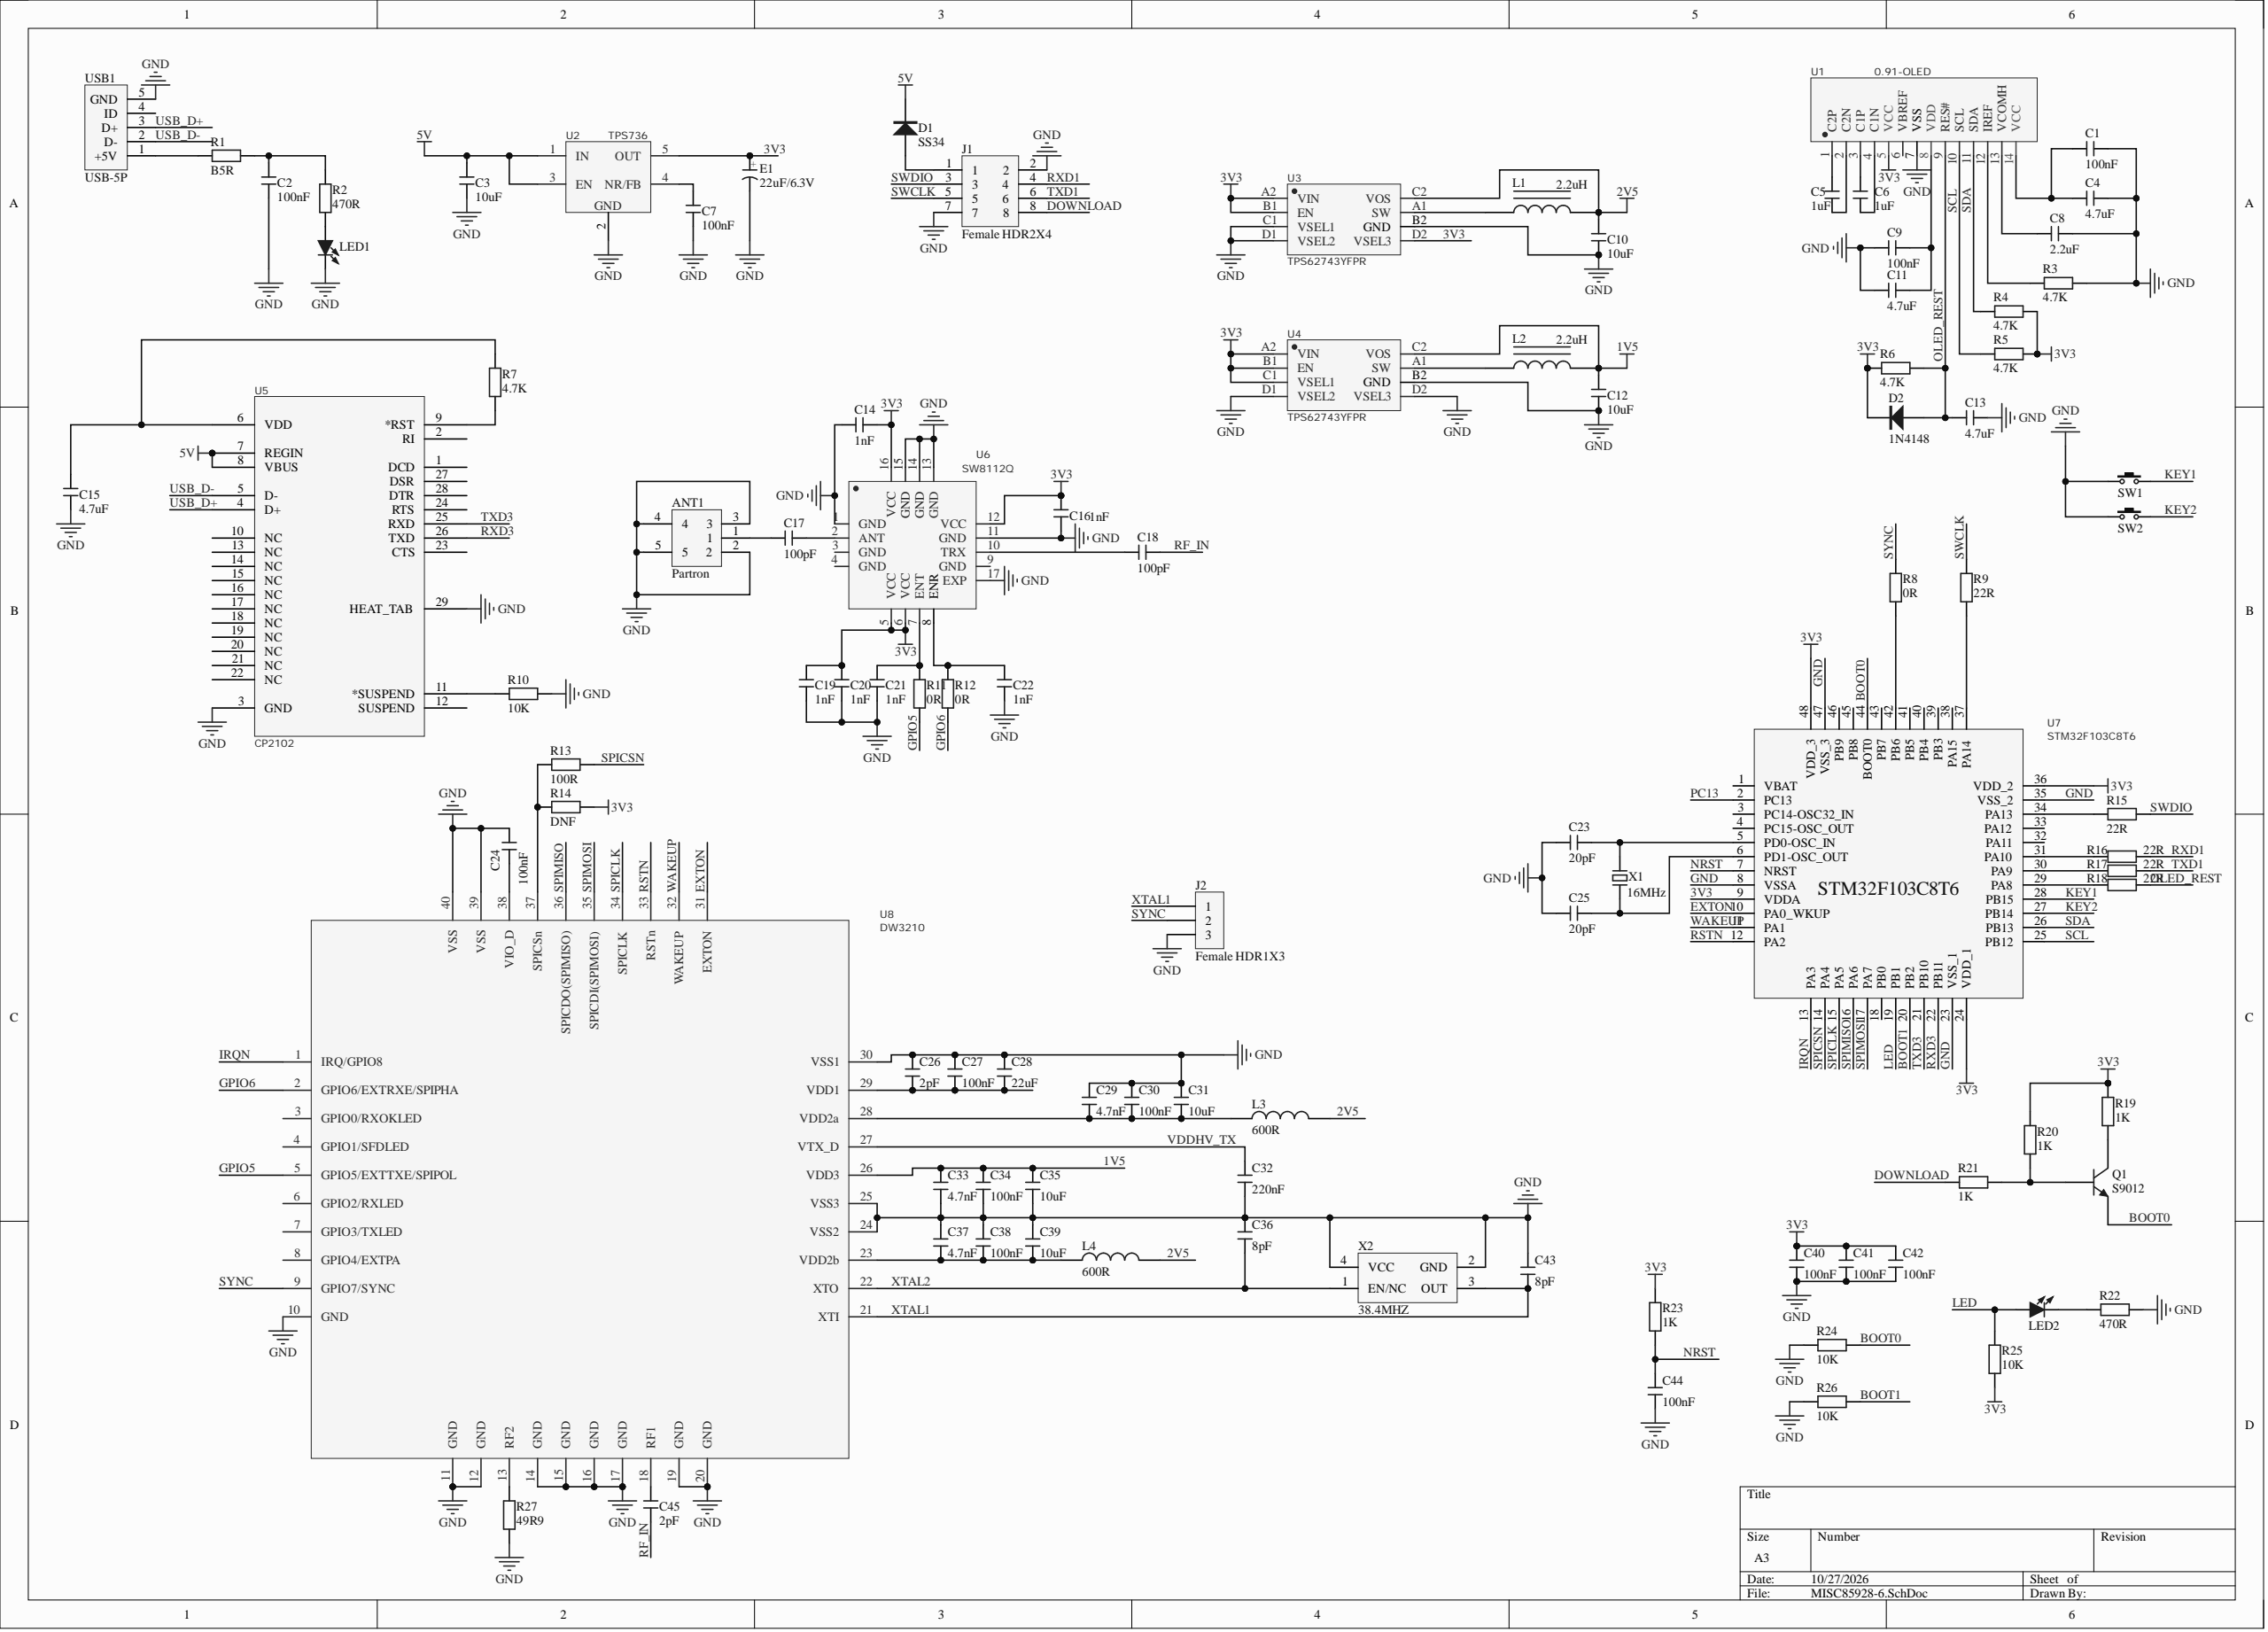Circuit board | Altium Designer | 98 parts | 79 nets
Bill of materials:
Comment,Description,Designator,Footprint,LibRef,Quantity
"Partron","","ANT1","天线座5p","Partron","1"
"100nF","Chip capacitor","C1, C2, C7, C9, C24, C27, C30, C34, C38, C40, C41, C42, C44","C 0603_L","C","13"
"10uF","Chip capacitor","C3, C10, C12, C31, C35, C39","C 0603_L","C","6"
"4.7uF","Chip capacitor","C4, C11, C13, C15","C 0603_L","C","4"
"1uF","Chip capacitor","C5, C6","C 0603_L","C","2"
"2.2uF","Chip capacitor","C8","C 0603_L","C","1"
"1nF","Chip capacitor","C14, C16, C19, C20, C21, C22","C 0603_L","C","6"
"100pF","Chip capacitor","C17, C18","C 0603_L","C","2"
"20pF","Chip capacitor","C23, C25","C 0603_L","C","2"
"2pF","Chip capacitor","C26, C45","C 0603_L","C","2"
"22uF","Chip capacitor","C28","C 0603_L","C","1"
"4.7nF","Chip capacitor","C29, C33, C37","C 0603_L","C","3"
"220nF","Chip capacitor","C32","C 0603_L","C","1"
"8pF","Chip capacitor","C36, C43","C 0603_L","C","2"
"SS34","Switching diode","D1","MINI_MELF (LL34)","1N4148","1"
"1N4148","Switching diode","D2","MINI_MELF (LL34)","1N4148","1"
"22uF/6.3V","Chip tantalum capacitor","E1","C 0603_L","CT","1"
"Female HDR2X4","","J1","Fe-HDR2X4/2.54-S","Female HDR2X4","1"
"Female HDR1X3","","J2","Fe-HDR1X3/2.54-S","Female HDR1X3","1"
"Inductor Iron","Magnetic-Core Inductor","L1, L2","L 0603","Inductor Iron","2"
"600R","Low-power chip inductor","L3, L4","L 0603","L","2"
"Red","Chip LED","LED1, LED2","LED 0805G","LED-SMD","2"
"S9012","NPN Bipolar Transistor","Q1","SOT-23B_N","QNPN","1"
"B5R","Chip resistor","R1","R 0603_L","R","1"
"470R","Chip resistor","R2, R22","R 0603_L","R","2"
"4.7K","Chip resistor","R3, R4, R5, R6, R7","R 0603_L","R","5"
"0R","Chip resistor","R8, R11, R12","R 0603_L","R","3"
"22R","Chip resistor","R9, R15, R16, R17, R18","R 0603_L","R","5"
"10K","Chip resistor","R10, R24, R25, R26","R 0603_L","R","4"
"100R","Chip resistor","R13","R 0603_L","R","1"
"DNF","Chip resistor","R14","R 0603_L","R","1"
"1K","Chip resistor","R19, R20, R21, R23","R 0603_L","R","4"
"49R9","Chip resistor","R27","R 0603_L","R","1"
"3x6x5","3x6 tact switch","SW1, SW2","TSW SMD-3*6*2.5","TSW 3x6","2"
"0.91-OLED","","U1","OLED0.91","0.91-OLED","1"
"TPS736","","U2","SOT-23-5_L3.0-W1.7-P0.95-LS2.8-BR","TPS73633DBVR","1"
"TPS62743YFPR","","U3, U4","DSBGA-8_L1.6-W0.9-R2-C4-P0.40-BL","TPS62743YFPR","2"
"CP2102","","U5","CP2102","CP2102_1","1"
"SW8112Q","","U6","QFN-16_L3.0-W3.0-P0.50-BL-EP1.7","SW8112Q","1"
"STM32F103C8T6","","U7","LQFP48 7X7","STM32F103C8T6","1"
"DW3210","","U8","DW3210","DW3210","1"
"USB-5P","Micro USB female socket","USB1","USB-MICRO_A","USB-5P","1"
"16MHz","2-pin passive crystal","X1","OSC 3215-2P","XTAL-2P","1"
"38.4MHZ","4-pin active crystal oscillator","X2","OSC 1612-4P","XTAL-ACT-4P","1"
Netlist (Protel format):
[
ANT1
天线座5p
Partron



]
[
C1
C 0603_L
100nF



]
[
C2
C 0603_L
100nF



]
[
C3
C 0603_L
10uF



]
[
C4
C 0603_L
4.7uF



]
[
C5
C 0603_L
1uF



]
[
C6
C 0603_L
1uF



]
[
C7
C 0603_L
100nF



]
[
C8
C 0603_L
2.2uF



]
[
C9
C 0603_L
100nF



]
[
C10
C 0603_L
10uF



]
[
C11
C 0603_L
4.7uF



]
[
C12
C 0603_L
10uF



]
[
C13
C 0603_L
4.7uF



]
[
C14
C 0603_L
1nF



]
[
C15
C 0603_L
4.7uF



]
[
C16
C 0603_L
1nF



]
[
C17
C 0603_L
100pF



]
[
C18
C 0603_L
100pF



]
[
C19
C 0603_L
1nF



]
[
C20
C 0603_L
1nF



]
[
C21
C 0603_L
1nF



]
[
C22
C 0603_L
1nF



]
[
C23
C 0603_L
20pF



]
[
C24
C 0603_L
100nF



]
[
C25
C 0603_L
20pF



]
[
C26
C 0603_L
2pF



]
[
C27
C 0603_L
100nF



]
[
C28
C 0603_L
22uF



]
[
C29
C 0603_L
4.7nF



]
[
C30
C 0603_L
100nF



]
[
C31
C 0603_L
10uF



]
[
C32
C 0603_L
220nF



]
[
C33
C 0603_L
4.7nF



]
[
C34
C 0603_L
100nF



]
[
C35
C 0603_L
10uF



]
[
C36
C 0603_L
8pF



]
[
C37
C 0603_L
4.7nF



]
[
C38
C 0603_L
100nF



]
[
C39
C 0603_L
10uF



]
[
C40
C 0603_L
100nF



]
[
C41
C 0603_L
100nF



]
[
C42
C 0603_L
100nF



]
[
C43
C 0603_L
8pF



]
[
C44
C 0603_L
100nF



]
[
C45
C 0603_L
2pF



]
[
D1
MINI_MELF (LL34)
SS34



]
[
D2
MINI_MELF (LL34)
1N4148



]
[
E1
C 0603_L
22uF/6.3V



]
[
J1
Fe-HDR2X4/2.54-S
Female HDR2X4



]
[
J2
Fe-HDR1X3/2.54-S
Female HDR1X3



]
[
L1
L 0603
Inductor Iron



]
[
L2
L 0603
Inductor Iron



]
[
L3
L 0603
600R



]
[
L4
L 0603
600R



]
[
LED1
LED 0805G
Red



]
[
LED2
LED 0805G
Red



]
[
Q1
SOT-23B_N
S9012



]
[
R1
R 0603_L
B5R



]
[
R2
R 0603_L
470R



]
[
R3
R 0603_L
4.7K



]
[
R4
R 0603_L
4.7K



]
[
R5
R 0603_L
4.7K



]
[
R6
R 0603_L
4.7K



]
[
R7
R 0603_L
4.7K



]
[
R8
R 0603_L
0R



]
[
R9
R 0603_L
22R



]
[
R10
R 0603_L
10K



]
[
R11
R 0603_L
0R



]
[
R12
R 0603_L
0R



]
[
R13
R 0603_L
100R



]
[
R14
R 0603_L
DNF



]
[
R15
R 0603_L
22R



]
[
R16
R 0603_L
22R



]
[
R17
R 0603_L
22R



]
[
R18
R 0603_L
22R



]
[
R19
R 0603_L
1K



]
[
R20
R 0603_L
1K



]
[
R21
R 0603_L
1K



]
[
R22
R 0603_L
470R



]
[
R23
R 0603_L
1K



]
[
R24
R 0603_L
10K



]
[
R25
R 0603_L
10K



]
[
R26
R 0603_L
10K



]
[
R27
R 0603_L
49R9



]
[
SW1
TSW SMD-3*6*2.5
3x6x5



]
[
SW2
TSW SMD-3*6*2.5
3x6x5



]
[
U1
OLED0.91
0.91-OLED



]
[
U2
SOT-23-5_L3.0-W1.7-P0.95-LS2.8-BR
TPS736



]
[
U3
DSBGA-8_L1.6-W0.9-R2-C4-P0.40-BL
TPS62743YFPR



]
[
U4
DSBGA-8_L1.6-W0.9-R2-C4-P0.40-BL
TPS62743YFPR



]
[
U5
CP2102
CP2102



]
[
U6
QFN-16_L3.0-W3.0-P0.50-BL-EP1.7
SW8112Q



]
[
U7
LQFP48 7X7
STM32F103C8T6



]
[
U8
DW3210
DW3210



]
[
USB1
USB-MICRO_A
USB-5P



]
[
X1
OSC 3215-2P
16MHz



]
[
X2
OSC 1612-4P
38.4MHZ



]
(
XTAL2
C36-2
U8-22
X2-1
)
(
XTAL1
C43-2
J2-1
U8-21
X2-3
)
(
WAKEUP
U7-11
U8-32
)
(
VDDHV_TX
C32-1
U8-27
)
(
USB_D-
U5-5
USB1-2
)
(
USB_D+
U5-4
USB1-3
)
(
TXD3
U5-25
U7-21
)
(
TXD1
J1-6
R17-1
)
(
SYNC
J2-2
R8-2
U8-9
)
(
SWDIO
J1-3
R15-1
)
(
SWCLK
J1-5
R9-2
)
(
SPIMOSI
U7-17
U8-35
)
(
SPIMISO
U7-16
U8-36
)
(
SPICSN
R13-1
U7-14
)
(
SPICLK
U7-15
U8-34
)
(
SDA
R4-2
U1-11
U7-26
)
(
SCL
R5-2
U1-10
U7-25
)
(
RXD3
U5-26
U7-22
)
(
RXD1
J1-4
R16-1
)
(
RSTN
U7-12
U8-33
)
(
RF_IN
C18-1
C45-2
)
(
OLED_REST
C13-2
D2-1
R6-1
R18-1
U1-9
)
(
NRST
C44-1
R23-1
U7-7
)
(
NetR27_2
R27-2
U8-13
)
(
NetR18_2
R18-2
U7-29
)
(
NetR17_2
R17-2
U7-30
)
(
NetR16_2
R16-2
U7-31
)
(
NetR15_2
R15-2
U7-34
)
(
NetR13_2
R13-2
R14-2
U8-37
)
(
NetR10_2
R10-2
U5-11
)
(
NetR9_1
R9-1
U7-37
)
(
NetR8_1
R8-1
U7-42
)
(
NetR7_1
R7-1
U5-9
)
(
NetR3_2
R3-2
U1-12
)
(
NetR1_1
R1-1
USB1-1
)
(
NetQ1_2
Q1-2
R20-2
R21-2
)
(
NetQ1_1
Q1-1
R19-2
)
(
NetLED2_2
LED2-2
R22-1
)
(
NetLED1_1
LED1-1
R2-1
)
(
NetL2_1
L2-1
U4-A1
)
(
NetL1_1
L1-1
U3-A1
)
(
NetD1_1
D1-1
J1-1
)
(
NetC45_1
C45-1
U8-18
)
(
NetC37_2
C37-2
C38-2
C39-2
L4-1
U8-23
)
(
NetC29_2
C29-2
C30-2
C31-2
L3-1
U8-28
)
(
NetC26_2
C26-2
C27-2
C28-2
U8-29
)
(
NetC25_2
C25-2
U7-6
X1-1
)
(
NetC24_2
C24-2
U8-38
)
(
NetC23_2
C23-2
U7-5
X1-2
)
(
NetC22_1
C22-1
R12-2
U6-8
)
(
NetC21_1
C21-1
R11-2
U6-7
)
(
NetC18_2
C18-2
U6-10
)
(
NetC17_1
C17-1
U6-2
)
(
NetC15_2
C15-2
R7-2
U5-6
)
(
NetC9_1
C9-1
C11-1
U1-8
)
(
NetC8_2
C8-2
U1-13
)
(
NetC7_2
C7-2
U2-4
)
(
NetC6_2
C6-2
U1-3
)
(
NetC6_1
C6-1
U1-4
)
(
NetC5_2
C5-2
U1-1
)
(
NetC5_1
C5-1
U1-2
)
(
NetC2_2
C2-2
R1-2
R2-2
)
(
NetC1_2
C1-2
C4-2
U1-14
)
(
NetANT1_1
ANT1-1
C17-2
)
(
LED
LED2-1
R25-1
U7-19
)
(
KEY2
SW2-2
U7-27
)
(
KEY1
SW1-2
U7-28
)
(
IRQN
U7-13
U8-1
)
(
GPIO6
R12-1
U8-2
)
(
GPIO5
R11-1
U8-5
)
(
GND
ANT1-2
ANT1-3
ANT1-4
ANT1-5
C1-1
C2-1
C3-1
C4-1
C7-1
C8-1
C9-2
C10-1
C11-2
C12-1
C13-1
C14-2
C15-1
C16-2
C19-2
C20-2
C21-2
C22-2
C23-1
C24-1
C25-1
C26-1
C27-1
C28-1
C29-1
C30-1
C31-1
C32-2
C33-2
C34-2
C35-2
C36-1
C37-1
C38-1
C39-1
C40-2
C41-2
C42-2
C43-1
C44-2
E1-2
J1-2
J1-7
J2-3
LED1-2
R3-1
R10-1
R22-2
R24-2
R26-2
R27-1
SW1-1
SW2-1
U1-7
U2-2
U3-B2
U3-C1
U3-D1
U4-B2
U4-D1
U4-D2
U5-3
U5-29
U6-1
U6-11
U6-13
U6-14
U6-15
U6-17
U7-8
U7-23
U7-35
U7-47
U8-10
U8-11
U8-12
U8-14
U8-15
U8-16
U8-17
U8-19
U8-20
U8-24
U8-25
U8-30
U8-39
U8-40
USB1-5
X2-2
X2-4
)
(
EXTON
U7-10
U8-31
)
(
DOWNLOAD
J1-8
R21-1
)
(
BOOT1
R26-1
U7-20
)
(
BOOT0
Q1-3
R24-1
U7-44
)
(
5V
C3-2
D1-2
U2-1
U2-3
U5-7
U5-8
)
(
3V3
C14-1
C16-1
C19-1
C20-1
C40-1
C41-1
C42-1
D2-2
E1-1
R4-1
R5-1
R6-2
R14-1
R19-1
R20-1
R23-2
R25-2
U1-5
U2-5
U3-A2
U3-B1
U3-D2
U4-A2
U4-B1
U4-C1
U6-5
U6-6
U6-12
U6-16
U7-9
U7-24
U7-36
U7-48
)
(
2V5
C10-2
L1-2
L3-2
L4-2
U3-C2
)
(
1V5
C12-2
C33-1
C34-1
C35-1
L2-2
U4-C2
U8-26
)